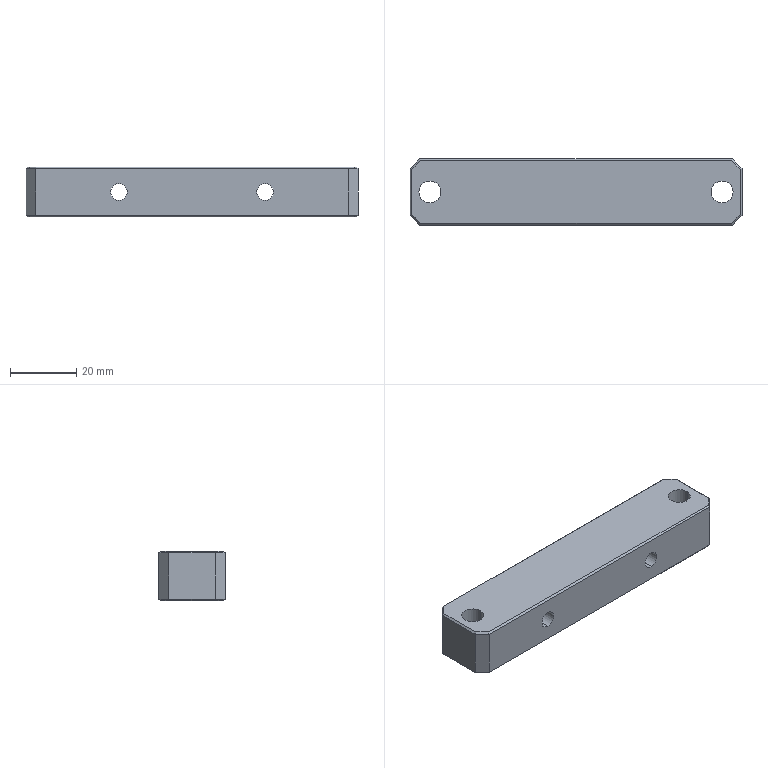Part | SolidWorks | features Chamfer 2, HoleWzd 2, Extrusion 1 | 1 solid | 40 faces | box 100 x 20 x 15 mm | volume 27033 mm3 | plane 28 | cylinder 12 | commonest cylinder face diameters 5 x4 6.6 x4 11 x4
STEP:
#1=CARTESIAN_POINT('',(22.,20.,10.));
#2=VERTEX_POINT('',#1);
#3=CARTESIAN_POINT('',(22.,20.,5.));
#4=VERTEX_POINT('',#3);
#5=CARTESIAN_POINT('',(22.,20.,7.5));
#6=DIRECTION('',(0.,-1.,0.));
#7=DIRECTION('',(0.,0.,-1.));
#8=AXIS2_PLACEMENT_3D('',#5,#6,#7);
#9=CIRCLE('',#8,2.5);
#10=EDGE_CURVE('',#2,#4,#9,.T.);
#11=ORIENTED_EDGE('',*,*,#10,.F.);
#12=CARTESIAN_POINT('',(22.,0.,10.));
#13=VERTEX_POINT('',#12);
#14=CARTESIAN_POINT('',(22.,0.,10.));
#15=DIRECTION('',(0.,-1.,0.));
#16=VECTOR('',#15,1000.);
#17=LINE('',#14,#16);
#18=EDGE_CURVE('',#2,#13,#17,.T.);
#19=ORIENTED_EDGE('',*,*,#18,.T.);
#20=CARTESIAN_POINT('',(22.,0.,5.));
#21=VERTEX_POINT('',#20);
#22=CARTESIAN_POINT('',(22.,0.,7.5));
#23=DIRECTION('',(0.,-1.,0.));
#24=DIRECTION('',(0.,0.,-1.));
#25=AXIS2_PLACEMENT_3D('',#22,#23,#24);
#26=CIRCLE('',#25,2.5);
#27=EDGE_CURVE('',#13,#21,#26,.T.);
#28=ORIENTED_EDGE('',*,*,#27,.T.);
#29=CARTESIAN_POINT('',(22.,0.,5.));
#30=DIRECTION('',(0.,-1.,0.));
#31=VECTOR('',#30,1000.);
#32=LINE('',#29,#31);
#33=EDGE_CURVE('',#4,#21,#32,.T.);
#34=ORIENTED_EDGE('',*,*,#33,.F.);
#35=EDGE_LOOP('',(#11,#19,#28,#34));
#36=FACE_OUTER_BOUND('',#35,.T.);
#37=CARTESIAN_POINT('',(22.,0.,7.5));
#38=DIRECTION('',(0.,-1.,0.));
#39=DIRECTION('',(0.,0.,-1.));
#40=AXIS2_PLACEMENT_3D('',#37,#38,#39);
#41=CYLINDRICAL_SURFACE('',#40,2.5);
#42=ADVANCED_FACE('',(#36),#41,.F.);
#43=CARTESIAN_POINT('',(-22.,20.,10.));
#44=VERTEX_POINT('',#43);
#45=CARTESIAN_POINT('',(-22.,20.,5.));
#46=VERTEX_POINT('',#45);
#47=CARTESIAN_POINT('',(-22.,20.,7.5));
#48=DIRECTION('',(0.,-1.,0.));
#49=DIRECTION('',(0.,0.,-1.));
#50=AXIS2_PLACEMENT_3D('',#47,#48,#49);
#51=CIRCLE('',#50,2.5);
#52=EDGE_CURVE('',#44,#46,#51,.T.);
#53=ORIENTED_EDGE('',*,*,#52,.F.);
#54=CARTESIAN_POINT('',(-22.,0.,10.));
#55=VERTEX_POINT('',#54);
#56=CARTESIAN_POINT('',(-22.,0.,10.));
#57=DIRECTION('',(0.,-1.,0.));
#58=VECTOR('',#57,1000.);
#59=LINE('',#56,#58);
#60=EDGE_CURVE('',#44,#55,#59,.T.);
#61=ORIENTED_EDGE('',*,*,#60,.T.);
#62=CARTESIAN_POINT('',(-22.,0.,5.));
#63=VERTEX_POINT('',#62);
#64=CARTESIAN_POINT('',(-22.,0.,7.5));
#65=DIRECTION('',(0.,-1.,0.));
#66=DIRECTION('',(0.,0.,-1.));
#67=AXIS2_PLACEMENT_3D('',#64,#65,#66);
#68=CIRCLE('',#67,2.5);
#69=EDGE_CURVE('',#55,#63,#68,.T.);
#70=ORIENTED_EDGE('',*,*,#69,.T.);
#71=CARTESIAN_POINT('',(-22.,0.,5.));
#72=DIRECTION('',(0.,-1.,0.));
#73=VECTOR('',#72,1000.);
#74=LINE('',#71,#73);
#75=EDGE_CURVE('',#46,#63,#74,.T.);
#76=ORIENTED_EDGE('',*,*,#75,.F.);
#77=EDGE_LOOP('',(#53,#61,#70,#76));
#78=FACE_OUTER_BOUND('',#77,.T.);
#79=CARTESIAN_POINT('',(-22.,0.,7.5));
#80=DIRECTION('',(0.,-1.,0.));
#81=DIRECTION('',(0.,0.,-1.));
#82=AXIS2_PLACEMENT_3D('',#79,#80,#81);
#83=CYLINDRICAL_SURFACE('',#82,2.5);
#84=ADVANCED_FACE('',(#78),#83,.F.);
#85=CARTESIAN_POINT('',(-38.5,10.,6.8));
#86=VERTEX_POINT('',#85);
#87=CARTESIAN_POINT('',(-49.5,10.,6.8));
#88=VERTEX_POINT('',#87);
#89=CARTESIAN_POINT('',(-44.,10.,6.8));
#90=DIRECTION('',(0.,0.,-1.));
#91=DIRECTION('',(-1.,0.,0.));
#92=AXIS2_PLACEMENT_3D('',#89,#90,#91);
#93=CIRCLE('',#92,5.5);
#94=EDGE_CURVE('',#86,#88,#93,.T.);
#95=ORIENTED_EDGE('',*,*,#94,.F.);
#96=CARTESIAN_POINT('',(-38.5,10.,0.));
#97=VERTEX_POINT('',#96);
#98=CARTESIAN_POINT('',(-38.5,10.,0.));
#99=DIRECTION('',(0.,0.,-1.));
#100=VECTOR('',#99,1000.);
#101=LINE('',#98,#100);
#102=EDGE_CURVE('',#86,#97,#101,.T.);
#103=ORIENTED_EDGE('',*,*,#102,.T.);
#104=CARTESIAN_POINT('',(-49.5,10.,0.));
#105=VERTEX_POINT('',#104);
#106=CARTESIAN_POINT('',(-44.,10.,0.));
#107=DIRECTION('',(0.,0.,-1.));
#108=DIRECTION('',(-1.,0.,0.));
#109=AXIS2_PLACEMENT_3D('',#106,#107,#108);
#110=CIRCLE('',#109,5.5);
#111=EDGE_CURVE('',#97,#105,#110,.T.);
#112=ORIENTED_EDGE('',*,*,#111,.T.);
#113=CARTESIAN_POINT('',(-49.5,10.,0.));
#114=DIRECTION('',(0.,0.,-1.));
#115=VECTOR('',#114,1000.);
#116=LINE('',#113,#115);
#117=EDGE_CURVE('',#88,#105,#116,.T.);
#118=ORIENTED_EDGE('',*,*,#117,.F.);
#119=EDGE_LOOP('',(#95,#103,#112,#118));
#120=FACE_OUTER_BOUND('',#119,.T.);
#121=CARTESIAN_POINT('',(-44.,10.,0.));
#122=DIRECTION('',(0.,0.,-1.));
#123=DIRECTION('',(-1.,0.,0.));
#124=AXIS2_PLACEMENT_3D('',#121,#122,#123);
#125=CYLINDRICAL_SURFACE('',#124,5.5);
#126=ADVANCED_FACE('',(#120),#125,.F.);
#127=CARTESIAN_POINT('',(-40.7,10.,15.));
#128=VERTEX_POINT('',#127);
#129=CARTESIAN_POINT('',(-47.3,10.,15.));
#130=VERTEX_POINT('',#129);
#131=CARTESIAN_POINT('',(-44.,10.,15.));
#132=DIRECTION('',(0.,0.,-1.));
#133=DIRECTION('',(-1.,0.,0.));
#134=AXIS2_PLACEMENT_3D('',#131,#132,#133);
#135=CIRCLE('',#134,3.3);
#136=EDGE_CURVE('',#128,#130,#135,.T.);
#137=ORIENTED_EDGE('',*,*,#136,.F.);
#138=CARTESIAN_POINT('',(-40.7,10.,6.8));
#139=VERTEX_POINT('',#138);
#140=CARTESIAN_POINT('',(-40.7,10.,0.));
#141=DIRECTION('',(0.,0.,-1.));
#142=VECTOR('',#141,1000.);
#143=LINE('',#140,#142);
#144=EDGE_CURVE('',#128,#139,#143,.T.);
#145=ORIENTED_EDGE('',*,*,#144,.T.);
#146=CARTESIAN_POINT('',(-47.3,10.,6.8));
#147=VERTEX_POINT('',#146);
#148=CARTESIAN_POINT('',(-44.,10.,6.8));
#149=DIRECTION('',(0.,0.,-1.));
#150=DIRECTION('',(-1.,0.,0.));
#151=AXIS2_PLACEMENT_3D('',#148,#149,#150);
#152=CIRCLE('',#151,3.3);
#153=EDGE_CURVE('',#139,#147,#152,.T.);
#154=ORIENTED_EDGE('',*,*,#153,.T.);
#155=CARTESIAN_POINT('',(-47.3,10.,0.));
#156=DIRECTION('',(0.,0.,-1.));
#157=VECTOR('',#156,1000.);
#158=LINE('',#155,#157);
#159=EDGE_CURVE('',#130,#147,#158,.T.);
#160=ORIENTED_EDGE('',*,*,#159,.F.);
#161=EDGE_LOOP('',(#137,#145,#154,#160));
#162=FACE_OUTER_BOUND('',#161,.T.);
#163=CARTESIAN_POINT('',(-44.,10.,0.));
#164=DIRECTION('',(0.,0.,-1.));
#165=DIRECTION('',(-1.,0.,0.));
#166=AXIS2_PLACEMENT_3D('',#163,#164,#165);
#167=CYLINDRICAL_SURFACE('',#166,3.3);
#168=ADVANCED_FACE('',(#162),#167,.F.);
#169=CARTESIAN_POINT('',(49.5,10.,6.8));
#170=VERTEX_POINT('',#169);
#171=CARTESIAN_POINT('',(38.5,10.,6.8));
#172=VERTEX_POINT('',#171);
#173=CARTESIAN_POINT('',(44.,10.,6.8));
#174=DIRECTION('',(0.,0.,-1.));
#175=DIRECTION('',(-1.,0.,0.));
#176=AXIS2_PLACEMENT_3D('',#173,#174,#175);
#177=CIRCLE('',#176,5.5);
#178=EDGE_CURVE('',#170,#172,#177,.T.);
#179=ORIENTED_EDGE('',*,*,#178,.F.);
#180=CARTESIAN_POINT('',(49.5,10.,0.));
#181=VERTEX_POINT('',#180);
#182=CARTESIAN_POINT('',(49.5,10.,0.));
#183=DIRECTION('',(0.,0.,-1.));
#184=VECTOR('',#183,1000.);
#185=LINE('',#182,#184);
#186=EDGE_CURVE('',#170,#181,#185,.T.);
#187=ORIENTED_EDGE('',*,*,#186,.T.);
#188=CARTESIAN_POINT('',(38.5,10.,0.));
#189=VERTEX_POINT('',#188);
#190=CARTESIAN_POINT('',(44.,10.,0.));
#191=DIRECTION('',(0.,0.,-1.));
#192=DIRECTION('',(-1.,0.,0.));
#193=AXIS2_PLACEMENT_3D('',#190,#191,#192);
#194=CIRCLE('',#193,5.5);
#195=EDGE_CURVE('',#181,#189,#194,.T.);
#196=ORIENTED_EDGE('',*,*,#195,.T.);
#197=CARTESIAN_POINT('',(38.5,10.,0.));
#198=DIRECTION('',(0.,0.,-1.));
#199=VECTOR('',#198,1000.);
#200=LINE('',#197,#199);
#201=EDGE_CURVE('',#172,#189,#200,.T.);
#202=ORIENTED_EDGE('',*,*,#201,.F.);
#203=EDGE_LOOP('',(#179,#187,#196,#202));
#204=FACE_OUTER_BOUND('',#203,.T.);
#205=CARTESIAN_POINT('',(44.,10.,0.));
#206=DIRECTION('',(0.,0.,-1.));
#207=DIRECTION('',(-1.,0.,0.));
#208=AXIS2_PLACEMENT_3D('',#205,#206,#207);
#209=CYLINDRICAL_SURFACE('',#208,5.5);
#210=ADVANCED_FACE('',(#204),#209,.F.);
#211=CARTESIAN_POINT('',(47.3,10.,15.));
#212=VERTEX_POINT('',#211);
#213=CARTESIAN_POINT('',(40.7,10.,15.));
#214=VERTEX_POINT('',#213);
#215=CARTESIAN_POINT('',(44.,10.,15.));
#216=DIRECTION('',(0.,0.,-1.));
#217=DIRECTION('',(-1.,0.,0.));
#218=AXIS2_PLACEMENT_3D('',#215,#216,#217);
#219=CIRCLE('',#218,3.3);
#220=EDGE_CURVE('',#212,#214,#219,.T.);
#221=ORIENTED_EDGE('',*,*,#220,.F.);
#222=CARTESIAN_POINT('',(47.3,10.,6.8));
#223=VERTEX_POINT('',#222);
#224=CARTESIAN_POINT('',(47.3,10.,0.));
#225=DIRECTION('',(0.,0.,-1.));
#226=VECTOR('',#225,1000.);
#227=LINE('',#224,#226);
#228=EDGE_CURVE('',#212,#223,#227,.T.);
#229=ORIENTED_EDGE('',*,*,#228,.T.);
#230=CARTESIAN_POINT('',(40.7,10.,6.8));
#231=VERTEX_POINT('',#230);
#232=CARTESIAN_POINT('',(44.,10.,6.8));
#233=DIRECTION('',(0.,0.,-1.));
#234=DIRECTION('',(-1.,0.,0.));
#235=AXIS2_PLACEMENT_3D('',#232,#233,#234);
#236=CIRCLE('',#235,3.3);
#237=EDGE_CURVE('',#223,#231,#236,.T.);
#238=ORIENTED_EDGE('',*,*,#237,.T.);
#239=CARTESIAN_POINT('',(40.7,10.,0.));
#240=DIRECTION('',(0.,0.,-1.));
#241=VECTOR('',#240,1000.);
#242=LINE('',#239,#241);
#243=EDGE_CURVE('',#214,#231,#242,.T.);
#244=ORIENTED_EDGE('',*,*,#243,.F.);
#245=EDGE_LOOP('',(#221,#229,#238,#244));
#246=FACE_OUTER_BOUND('',#245,.T.);
#247=CARTESIAN_POINT('',(44.,10.,0.));
#248=DIRECTION('',(0.,0.,-1.));
#249=DIRECTION('',(-1.,0.,0.));
#250=AXIS2_PLACEMENT_3D('',#247,#248,#249);
#251=CYLINDRICAL_SURFACE('',#250,3.3);
#252=ADVANCED_FACE('',(#246),#251,.F.);
#253=CARTESIAN_POINT('',(-50.,3.,0.5));
#254=VERTEX_POINT('',#253);
#255=CARTESIAN_POINT('',(-50.,3.,14.5));
#256=VERTEX_POINT('',#255);
#257=CARTESIAN_POINT('',(-50.,3.,15.));
#258=DIRECTION('',(0.,0.,1.));
#259=VECTOR('',#258,1000.);
#260=LINE('',#257,#259);
#261=EDGE_CURVE('',#254,#256,#260,.T.);
#262=ORIENTED_EDGE('',*,*,#261,.T.);
#263=CARTESIAN_POINT('',(-50.,17.,14.5));
#264=VERTEX_POINT('',#263);
#265=CARTESIAN_POINT('',(-50.,17.,14.5));
#266=DIRECTION('',(0.,1.,0.));
#267=VECTOR('',#266,1000.);
#268=LINE('',#265,#267);
#269=EDGE_CURVE('',#256,#264,#268,.T.);
#270=ORIENTED_EDGE('',*,*,#269,.T.);
#271=CARTESIAN_POINT('',(-50.,17.,0.5));
#272=VERTEX_POINT('',#271);
#273=CARTESIAN_POINT('',(-50.,17.,15.));
#274=DIRECTION('',(0.,0.,-1.));
#275=VECTOR('',#274,1000.);
#276=LINE('',#273,#275);
#277=EDGE_CURVE('',#264,#272,#276,.T.);
#278=ORIENTED_EDGE('',*,*,#277,.T.);
#279=CARTESIAN_POINT('',(-50.,20.,0.5));
#280=DIRECTION('',(0.,-1.,0.));
#281=VECTOR('',#280,1000.);
#282=LINE('',#279,#281);
#283=EDGE_CURVE('',#272,#254,#282,.T.);
#284=ORIENTED_EDGE('',*,*,#283,.T.);
#285=EDGE_LOOP('',(#262,#270,#278,#284));
#286=FACE_OUTER_BOUND('',#285,.T.);
#287=CARTESIAN_POINT('',(-50.,20.,15.));
#288=DIRECTION('',(1.,0.,0.));
#289=DIRECTION('',(0.,0.,-1.));
#290=AXIS2_PLACEMENT_3D('',#287,#288,#289);
#291=PLANE('',#290);
#292=ADVANCED_FACE('',(#286),#291,.F.);
#293=CARTESIAN_POINT('',(22.,0.,7.5));
#294=DIRECTION('',(0.,-1.,0.));
#295=DIRECTION('',(0.,0.,-1.));
#296=AXIS2_PLACEMENT_3D('',#293,#294,#295);
#297=CIRCLE('',#296,2.5);
#298=EDGE_CURVE('',#21,#13,#297,.T.);
#299=ORIENTED_EDGE('',*,*,#298,.F.);
#300=ORIENTED_EDGE('',*,*,#27,.F.);
#301=EDGE_LOOP('',(#299,#300));
#302=FACE_BOUND('',#301,.T.);
#303=CARTESIAN_POINT('',(-22.,0.,7.5));
#304=DIRECTION('',(0.,-1.,0.));
#305=DIRECTION('',(0.,0.,-1.));
#306=AXIS2_PLACEMENT_3D('',#303,#304,#305);
#307=CIRCLE('',#306,2.5);
#308=EDGE_CURVE('',#63,#55,#307,.T.);
#309=ORIENTED_EDGE('',*,*,#308,.F.);
#310=ORIENTED_EDGE('',*,*,#69,.F.);
#311=EDGE_LOOP('',(#309,#310));
#312=FACE_BOUND('',#311,.T.);
#313=CARTESIAN_POINT('',(47.,0.,0.5));
#314=VERTEX_POINT('',#313);
#315=CARTESIAN_POINT('',(47.,0.,14.5));
#316=VERTEX_POINT('',#315);
#317=CARTESIAN_POINT('',(47.,0.,15.));
#318=DIRECTION('',(0.,0.,1.));
#319=VECTOR('',#318,1000.);
#320=LINE('',#317,#319);
#321=EDGE_CURVE('',#314,#316,#320,.T.);
#322=ORIENTED_EDGE('',*,*,#321,.T.);
#323=CARTESIAN_POINT('',(-47.,0.,14.5));
#324=VERTEX_POINT('',#323);
#325=CARTESIAN_POINT('',(-47.,0.,14.5));
#326=DIRECTION('',(-1.,0.,0.));
#327=VECTOR('',#326,1000.);
#328=LINE('',#325,#327);
#329=EDGE_CURVE('',#316,#324,#328,.T.);
#330=ORIENTED_EDGE('',*,*,#329,.T.);
#331=CARTESIAN_POINT('',(-47.,0.,0.5));
#332=VERTEX_POINT('',#331);
#333=CARTESIAN_POINT('',(-47.,0.,15.));
#334=DIRECTION('',(0.,0.,-1.));
#335=VECTOR('',#334,1000.);
#336=LINE('',#333,#335);
#337=EDGE_CURVE('',#324,#332,#336,.T.);
#338=ORIENTED_EDGE('',*,*,#337,.T.);
#339=CARTESIAN_POINT('',(-50.,0.,0.5));
#340=DIRECTION('',(1.,0.,0.));
#341=VECTOR('',#340,1000.);
#342=LINE('',#339,#341);
#343=EDGE_CURVE('',#332,#314,#342,.T.);
#344=ORIENTED_EDGE('',*,*,#343,.T.);
#345=EDGE_LOOP('',(#322,#330,#338,#344));
#346=FACE_OUTER_BOUND('',#345,.T.);
#347=CARTESIAN_POINT('',(-50.,0.,15.));
#348=DIRECTION('',(0.,1.,0.));
#349=DIRECTION('',(0.,0.,1.));
#350=AXIS2_PLACEMENT_3D('',#347,#348,#349);
#351=PLANE('',#350);
#352=ADVANCED_FACE('',(#302,#312,#346),#351,.F.);
#353=CARTESIAN_POINT('',(50.,17.,0.5));
#354=VERTEX_POINT('',#353);
#355=CARTESIAN_POINT('',(50.,17.,14.5));
#356=VERTEX_POINT('',#355);
#357=CARTESIAN_POINT('',(50.,17.,15.));
#358=DIRECTION('',(0.,0.,1.));
#359=VECTOR('',#358,1000.);
#360=LINE('',#357,#359);
#361=EDGE_CURVE('',#354,#356,#360,.T.);
#362=ORIENTED_EDGE('',*,*,#361,.T.);
#363=CARTESIAN_POINT('',(50.,3.,14.5));
#364=VERTEX_POINT('',#363);
#365=CARTESIAN_POINT('',(50.,3.,14.5));
#366=DIRECTION('',(0.,-1.,0.));
#367=VECTOR('',#366,1000.);
#368=LINE('',#365,#367);
#369=EDGE_CURVE('',#356,#364,#368,.T.);
#370=ORIENTED_EDGE('',*,*,#369,.T.);
#371=CARTESIAN_POINT('',(50.,3.,0.5));
#372=VERTEX_POINT('',#371);
#373=CARTESIAN_POINT('',(50.,3.,15.));
#374=DIRECTION('',(0.,0.,-1.));
#375=VECTOR('',#374,1000.);
#376=LINE('',#373,#375);
#377=EDGE_CURVE('',#364,#372,#376,.T.);
#378=ORIENTED_EDGE('',*,*,#377,.T.);
#379=CARTESIAN_POINT('',(50.,20.,0.5));
#380=DIRECTION('',(0.,1.,0.));
#381=VECTOR('',#380,1000.);
#382=LINE('',#379,#381);
#383=EDGE_CURVE('',#372,#354,#382,.T.);
#384=ORIENTED_EDGE('',*,*,#383,.T.);
#385=EDGE_LOOP('',(#362,#370,#378,#384));
#386=FACE_OUTER_BOUND('',#385,.T.);
#387=CARTESIAN_POINT('',(50.,20.,15.));
#388=DIRECTION('',(-1.,0.,0.));
#389=DIRECTION('',(0.,0.,1.));
#390=AXIS2_PLACEMENT_3D('',#387,#388,#389);
#391=PLANE('',#390);
#392=ADVANCED_FACE('',(#386),#391,.F.);
#393=CARTESIAN_POINT('',(22.,20.,7.5));
#394=DIRECTION('',(0.,-1.,0.));
#395=DIRECTION('',(0.,0.,-1.));
#396=AXIS2_PLACEMENT_3D('',#393,#394,#395);
#397=CIRCLE('',#396,2.5);
#398=EDGE_CURVE('',#4,#2,#397,.T.);
#399=ORIENTED_EDGE('',*,*,#398,.T.);
#400=ORIENTED_EDGE('',*,*,#10,.T.);
#401=EDGE_LOOP('',(#399,#400));
#402=FACE_BOUND('',#401,.T.);
#403=CARTESIAN_POINT('',(-22.,20.,7.5));
#404=DIRECTION('',(0.,-1.,0.));
#405=DIRECTION('',(0.,0.,-1.));
#406=AXIS2_PLACEMENT_3D('',#403,#404,#405);
#407=CIRCLE('',#406,2.5);
#408=EDGE_CURVE('',#46,#44,#407,.T.);
#409=ORIENTED_EDGE('',*,*,#408,.T.);
#410=ORIENTED_EDGE('',*,*,#52,.T.);
#411=EDGE_LOOP('',(#409,#410));
#412=FACE_BOUND('',#411,.T.);
#413=CARTESIAN_POINT('',(-47.,20.,0.5));
#414=VERTEX_POINT('',#413);
#415=CARTESIAN_POINT('',(-47.,20.,14.5));
#416=VERTEX_POINT('',#415);
#417=CARTESIAN_POINT('',(-47.,20.,15.));
#418=DIRECTION('',(0.,0.,1.));
#419=VECTOR('',#418,1000.);
#420=LINE('',#417,#419);
#421=EDGE_CURVE('',#414,#416,#420,.T.);
#422=ORIENTED_EDGE('',*,*,#421,.T.);
#423=CARTESIAN_POINT('',(47.,20.,14.5));
#424=VERTEX_POINT('',#423);
#425=CARTESIAN_POINT('',(47.,20.,14.5));
#426=DIRECTION('',(1.,0.,0.));
#427=VECTOR('',#426,1000.);
#428=LINE('',#425,#427);
#429=EDGE_CURVE('',#416,#424,#428,.T.);
#430=ORIENTED_EDGE('',*,*,#429,.T.);
#431=CARTESIAN_POINT('',(47.,20.,0.5));
#432=VERTEX_POINT('',#431);
#433=CARTESIAN_POINT('',(47.,20.,15.));
#434=DIRECTION('',(0.,0.,-1.));
#435=VECTOR('',#434,1000.);
#436=LINE('',#433,#435);
#437=EDGE_CURVE('',#424,#432,#436,.T.);
#438=ORIENTED_EDGE('',*,*,#437,.T.);
#439=CARTESIAN_POINT('',(-50.,20.,0.5));
#440=DIRECTION('',(-1.,0.,0.));
#441=VECTOR('',#440,1000.);
#442=LINE('',#439,#441);
#443=EDGE_CURVE('',#432,#414,#442,.T.);
#444=ORIENTED_EDGE('',*,*,#443,.T.);
#445=EDGE_LOOP('',(#422,#430,#438,#444));
#446=FACE_OUTER_BOUND('',#445,.T.);
#447=CARTESIAN_POINT('',(-50.,20.,15.));
#448=DIRECTION('',(0.,-1.,0.));
#449=DIRECTION('',(1.,0.,0.));
#450=AXIS2_PLACEMENT_3D('',#447,#448,#449);
#451=PLANE('',#450);
#452=ADVANCED_FACE('',(#402,#412,#446),#451,.F.);
#453=CARTESIAN_POINT('',(49.5,3.207,15.));
#454=VERTEX_POINT('',#453);
#455=CARTESIAN_POINT('',(49.5,16.793,15.));
#456=VERTEX_POINT('',#455);
#457=CARTESIAN_POINT('',(49.5,17.,15.));
#458=DIRECTION('',(0.,1.,0.));
#459=VECTOR('',#458,1000.);
#460=LINE('',#457,#459);
#461=EDGE_CURVE('',#454,#456,#460,.T.);
#462=ORIENTED_EDGE('',*,*,#461,.T.);
#463=CARTESIAN_POINT('',(46.793,19.5,15.));
#464=VERTEX_POINT('',#463);
#465=CARTESIAN_POINT('',(33.146,33.146,15.));
#466=DIRECTION('',(-0.7071,0.7071,0.));
#467=VECTOR('',#466,1000.);
#468=LINE('',#465,#467);
#469=EDGE_CURVE('',#456,#464,#468,.T.);
#470=ORIENTED_EDGE('',*,*,#469,.T.);
#471=CARTESIAN_POINT('',(-46.793,19.5,15.));
#472=VERTEX_POINT('',#471);
#473=CARTESIAN_POINT('',(-47.,19.5,15.));
#474=DIRECTION('',(-1.,0.,0.));
#475=VECTOR('',#474,1000.);
#476=LINE('',#473,#475);
#477=EDGE_CURVE('',#464,#472,#476,.T.);
#478=ORIENTED_EDGE('',*,*,#477,.T.);
#479=CARTESIAN_POINT('',(-49.5,16.793,15.));
#480=VERTEX_POINT('',#479);
#481=CARTESIAN_POINT('',(-33.146,33.146,15.));
#482=DIRECTION('',(-0.7071,-0.7071,0.));
#483=VECTOR('',#482,1000.);
#484=LINE('',#481,#483);
#485=EDGE_CURVE('',#472,#480,#484,.T.);
#486=ORIENTED_EDGE('',*,*,#485,.T.);
#487=CARTESIAN_POINT('',(-49.5,3.207,15.));
#488=VERTEX_POINT('',#487);
#489=CARTESIAN_POINT('',(-49.5,3.,15.));
#490=DIRECTION('',(0.,-1.,0.));
#491=VECTOR('',#490,1000.);
#492=LINE('',#489,#491);
#493=EDGE_CURVE('',#480,#488,#492,.T.);
#494=ORIENTED_EDGE('',*,*,#493,.T.);
#495=CARTESIAN_POINT('',(-46.793,0.5,15.));
#496=VERTEX_POINT('',#495);
#497=CARTESIAN_POINT('',(-23.146,-23.146,15.));
#498=DIRECTION('',(0.7071,-0.7071,0.));
#499=VECTOR('',#498,1000.);
#500=LINE('',#497,#499);
#501=EDGE_CURVE('',#488,#496,#500,.T.);
#502=ORIENTED_EDGE('',*,*,#501,.T.);
#503=CARTESIAN_POINT('',(46.793,0.5,15.));
#504=VERTEX_POINT('',#503);
#505=CARTESIAN_POINT('',(47.,0.5,15.));
#506=DIRECTION('',(1.,0.,0.));
#507=VECTOR('',#506,1000.);
#508=LINE('',#505,#507);
#509=EDGE_CURVE('',#496,#504,#508,.T.);
#510=ORIENTED_EDGE('',*,*,#509,.T.);
#511=CARTESIAN_POINT('',(23.146,-23.146,15.));
#512=DIRECTION('',(0.7071,0.7071,0.));
#513=VECTOR('',#512,1000.);
#514=LINE('',#511,#513);
#515=EDGE_CURVE('',#504,#454,#514,.T.);
#516=ORIENTED_EDGE('',*,*,#515,.T.);
#517=EDGE_LOOP('',(#462,#470,#478,#486,#494,#502,#510,#516));
#518=FACE_OUTER_BOUND('',#517,.T.);
#519=CARTESIAN_POINT('',(-44.,10.,15.));
#520=DIRECTION('',(0.,0.,-1.));
#521=DIRECTION('',(-1.,0.,0.));
#522=AXIS2_PLACEMENT_3D('',#519,#520,#521);
#523=CIRCLE('',#522,3.3);
#524=EDGE_CURVE('',#130,#128,#523,.T.);
#525=ORIENTED_EDGE('',*,*,#524,.T.);
#526=ORIENTED_EDGE('',*,*,#136,.T.);
#527=EDGE_LOOP('',(#525,#526));
#528=FACE_BOUND('',#527,.T.);
#529=CARTESIAN_POINT('',(44.,10.,15.));
#530=DIRECTION('',(0.,0.,-1.));
#531=DIRECTION('',(-1.,0.,0.));
#532=AXIS2_PLACEMENT_3D('',#529,#530,#531);
#533=CIRCLE('',#532,3.3);
#534=EDGE_CURVE('',#214,#212,#533,.T.);
#535=ORIENTED_EDGE('',*,*,#534,.T.);
#536=ORIENTED_EDGE('',*,*,#220,.T.);
#537=EDGE_LOOP('',(#535,#536));
#538=FACE_BOUND('',#537,.T.);
#539=CARTESIAN_POINT('',(0.,0.,15.));
#540=DIRECTION('',(0.,0.,1.));
#541=DIRECTION('',(1.,0.,0.));
#542=AXIS2_PLACEMENT_3D('',#539,#540,#541);
#543=PLANE('',#542);
#544=ADVANCED_FACE('',(#518,#528,#538),#543,.T.);
#545=CARTESIAN_POINT('',(-46.793,0.5,0.));
#546=VERTEX_POINT('',#545);
#547=CARTESIAN_POINT('',(-49.5,3.207,0.));
#548=VERTEX_POINT('',#547);
#549=CARTESIAN_POINT('',(-49.646,3.354,0.));
#550=DIRECTION('',(-0.7071,0.7071,0.));
#551=VECTOR('',#550,1000.);
#552=LINE('',#549,#551);
#553=EDGE_CURVE('',#546,#548,#552,.T.);
#554=ORIENTED_EDGE('',*,*,#553,.T.);
#555=CARTESIAN_POINT('',(-49.5,0.,0.));
#556=DIRECTION('',(0.,1.,0.));
#557=VECTOR('',#556,1000.);
#558=LINE('',#555,#557);
#559=EDGE_CURVE('',#548,#105,#558,.T.);
#560=ORIENTED_EDGE('',*,*,#559,.T.);
#561=ORIENTED_EDGE('',*,*,#111,.F.);
#562=CARTESIAN_POINT('',(-44.,10.,0.));
#563=DIRECTION('',(0.,0.,-1.));
#564=DIRECTION('',(-1.,0.,0.));
#565=AXIS2_PLACEMENT_3D('',#562,#563,#564);
#566=CIRCLE('',#565,5.5);
#567=EDGE_CURVE('',#105,#97,#566,.T.);
#568=ORIENTED_EDGE('',*,*,#567,.F.);
#569=CARTESIAN_POINT('',(-49.5,16.793,0.));
#570=VERTEX_POINT('',#569);
#571=CARTESIAN_POINT('',(-49.5,0.,0.));
#572=DIRECTION('',(0.,1.,0.));
#573=VECTOR('',#572,1000.);
#574=LINE('',#571,#573);
#575=EDGE_CURVE('',#105,#570,#574,.T.);
#576=ORIENTED_EDGE('',*,*,#575,.T.);
#577=CARTESIAN_POINT('',(-46.793,19.5,0.));
#578=VERTEX_POINT('',#577);
#579=CARTESIAN_POINT('',(-46.646,19.646,0.));
#580=DIRECTION('',(0.7071,0.7071,0.));
#581=VECTOR('',#580,1000.);
#582=LINE('',#579,#581);
#583=EDGE_CURVE('',#570,#578,#582,.T.);
#584=ORIENTED_EDGE('',*,*,#583,.T.);
#585=CARTESIAN_POINT('',(46.793,19.5,0.));
#586=VERTEX_POINT('',#585);
#587=CARTESIAN_POINT('',(0.,19.5,0.));
#588=DIRECTION('',(1.,0.,0.));
#589=VECTOR('',#588,1000.);
#590=LINE('',#587,#589);
#591=EDGE_CURVE('',#578,#586,#590,.T.);
#592=ORIENTED_EDGE('',*,*,#591,.T.);
#593=CARTESIAN_POINT('',(49.5,16.793,0.));
#594=VERTEX_POINT('',#593);
#595=CARTESIAN_POINT('',(49.646,16.646,0.));
#596=DIRECTION('',(0.7071,-0.7071,0.));
#597=VECTOR('',#596,1000.);
#598=LINE('',#595,#597);
#599=EDGE_CURVE('',#586,#594,#598,.T.);
#600=ORIENTED_EDGE('',*,*,#599,.T.);
#601=CARTESIAN_POINT('',(49.5,0.,0.));
#602=DIRECTION('',(0.,-1.,0.));
#603=VECTOR('',#602,1000.);
#604=LINE('',#601,#603);
#605=EDGE_CURVE('',#594,#181,#604,.T.);
#606=ORIENTED_EDGE('',*,*,#605,.T.);
#607=CARTESIAN_POINT('',(44.,10.,0.));
#608=DIRECTION('',(0.,0.,-1.));
#609=DIRECTION('',(-1.,0.,0.));
#610=AXIS2_PLACEMENT_3D('',#607,#608,#609);
#611=CIRCLE('',#610,5.5);
#612=EDGE_CURVE('',#189,#181,#611,.T.);
#613=ORIENTED_EDGE('',*,*,#612,.F.);
#614=ORIENTED_EDGE('',*,*,#195,.F.);
#615=CARTESIAN_POINT('',(49.5,3.207,0.));
#616=VERTEX_POINT('',#615);
#617=CARTESIAN_POINT('',(49.5,0.,0.));
#618=DIRECTION('',(0.,-1.,0.));
#619=VECTOR('',#618,1000.);
#620=LINE('',#617,#619);
#621=EDGE_CURVE('',#181,#616,#620,.T.);
#622=ORIENTED_EDGE('',*,*,#621,.T.);
#623=CARTESIAN_POINT('',(46.793,0.5,0.));
#624=VERTEX_POINT('',#623);
#625=CARTESIAN_POINT('',(46.646,0.3536,0.));
#626=DIRECTION('',(-0.7071,-0.7071,0.));
#627=VECTOR('',#626,1000.);
#628=LINE('',#625,#627);
#629=EDGE_CURVE('',#616,#624,#628,.T.);
#630=ORIENTED_EDGE('',*,*,#629,.T.);
#631=CARTESIAN_POINT('',(0.,0.5,0.));
#632=DIRECTION('',(-1.,0.,0.));
#633=VECTOR('',#632,1000.);
#634=LINE('',#631,#633);
#635=EDGE_CURVE('',#624,#546,#634,.T.);
#636=ORIENTED_EDGE('',*,*,#635,.T.);
#637=EDGE_LOOP('',(#554,#560,#561,#568,#576,#584,#592,#600,#606,#613,#614,#622,#630,#636));
#638=FACE_OUTER_BOUND('',#637,.T.);
#639=CARTESIAN_POINT('',(0.,0.,0.));
#640=DIRECTION('',(0.,0.,1.));
#641=DIRECTION('',(1.,0.,0.));
#642=AXIS2_PLACEMENT_3D('',#639,#640,#641);
#643=PLANE('',#642);
#644=ADVANCED_FACE('',(#638),#643,.F.);
#645=ORIENTED_EDGE('',*,*,#228,.F.);
#646=ORIENTED_EDGE('',*,*,#534,.F.);
#647=ORIENTED_EDGE('',*,*,#243,.T.);
#648=CARTESIAN_POINT('',(44.,10.,6.8));
#649=DIRECTION('',(0.,0.,-1.));
#650=DIRECTION('',(-1.,0.,0.));
#651=AXIS2_PLACEMENT_3D('',#648,#649,#650);
#652=CIRCLE('',#651,3.3);
#653=EDGE_CURVE('',#231,#223,#652,.T.);
#654=ORIENTED_EDGE('',*,*,#653,.T.);
#655=EDGE_LOOP('',(#645,#646,#647,#654));
#656=FACE_OUTER_BOUND('',#655,.T.);
#657=CARTESIAN_POINT('',(44.,10.,0.));
#658=DIRECTION('',(0.,0.,-1.));
#659=DIRECTION('',(-1.,0.,0.));
#660=AXIS2_PLACEMENT_3D('',#657,#658,#659);
#661=CYLINDRICAL_SURFACE('',#660,3.3);
#662=ADVANCED_FACE('',(#656),#661,.F.);
#663=ORIENTED_EDGE('',*,*,#653,.F.);
#664=ORIENTED_EDGE('',*,*,#237,.F.);
#665=EDGE_LOOP('',(#663,#664));
#666=FACE_BOUND('',#665,.T.);
#667=CARTESIAN_POINT('',(44.,10.,6.8));
#668=DIRECTION('',(0.,0.,-1.));
#669=DIRECTION('',(-1.,0.,0.));
#670=AXIS2_PLACEMENT_3D('',#667,#668,#669);
#671=CIRCLE('',#670,5.5);
#672=EDGE_CURVE('',#172,#170,#671,.T.);
#673=ORIENTED_EDGE('',*,*,#672,.T.);
#674=ORIENTED_EDGE('',*,*,#178,.T.);
#675=EDGE_LOOP('',(#673,#674));
#676=FACE_OUTER_BOUND('',#675,.T.);
#677=CARTESIAN_POINT('',(47.3,10.,6.8));
#678=DIRECTION('',(0.,0.,1.));
#679=DIRECTION('',(1.,0.,0.));
#680=AXIS2_PLACEMENT_3D('',#677,#678,#679);
#681=PLANE('',#680);
#682=ADVANCED_FACE('',(#666,#676),#681,.F.);
#683=ORIENTED_EDGE('',*,*,#186,.F.);
#684=ORIENTED_EDGE('',*,*,#672,.F.);
#685=ORIENTED_EDGE('',*,*,#201,.T.);
#686=ORIENTED_EDGE('',*,*,#612,.T.);
#687=EDGE_LOOP('',(#683,#684,#685,#686));
#688=FACE_OUTER_BOUND('',#687,.T.);
#689=CARTESIAN_POINT('',(44.,10.,0.));
#690=DIRECTION('',(0.,0.,-1.));
#691=DIRECTION('',(-1.,0.,0.));
#692=AXIS2_PLACEMENT_3D('',#689,#690,#691);
#693=CYLINDRICAL_SURFACE('',#692,5.5);
#694=ADVANCED_FACE('',(#688),#693,.F.);
#695=ORIENTED_EDGE('',*,*,#144,.F.);
#696=ORIENTED_EDGE('',*,*,#524,.F.);
#697=ORIENTED_EDGE('',*,*,#159,.T.);
#698=CARTESIAN_POINT('',(-44.,10.,6.8));
#699=DIRECTION('',(0.,0.,-1.));
#700=DIRECTION('',(-1.,0.,0.));
#701=AXIS2_PLACEMENT_3D('',#698,#699,#700);
#702=CIRCLE('',#701,3.3);
#703=EDGE_CURVE('',#147,#139,#702,.T.);
#704=ORIENTED_EDGE('',*,*,#703,.T.);
#705=EDGE_LOOP('',(#695,#696,#697,#704));
#706=FACE_OUTER_BOUND('',#705,.T.);
#707=CARTESIAN_POINT('',(-44.,10.,0.));
#708=DIRECTION('',(0.,0.,-1.));
#709=DIRECTION('',(-1.,0.,0.));
#710=AXIS2_PLACEMENT_3D('',#707,#708,#709);
#711=CYLINDRICAL_SURFACE('',#710,3.3);
#712=ADVANCED_FACE('',(#706),#711,.F.);
#713=ORIENTED_EDGE('',*,*,#703,.F.);
#714=ORIENTED_EDGE('',*,*,#153,.F.);
#715=EDGE_LOOP('',(#713,#714));
#716=FACE_BOUND('',#715,.T.);
#717=CARTESIAN_POINT('',(-44.,10.,6.8));
#718=DIRECTION('',(0.,0.,-1.));
#719=DIRECTION('',(-1.,0.,0.));
#720=AXIS2_PLACEMENT_3D('',#717,#718,#719);
#721=CIRCLE('',#720,5.5);
#722=EDGE_CURVE('',#88,#86,#721,.T.);
#723=ORIENTED_EDGE('',*,*,#722,.T.);
#724=ORIENTED_EDGE('',*,*,#94,.T.);
#725=EDGE_LOOP('',(#723,#724));
#726=FACE_OUTER_BOUND('',#725,.T.);
#727=CARTESIAN_POINT('',(-40.7,10.,6.8));
#728=DIRECTION('',(0.,0.,1.));
#729=DIRECTION('',(1.,0.,0.));
#730=AXIS2_PLACEMENT_3D('',#727,#728,#729);
#731=PLANE('',#730);
#732=ADVANCED_FACE('',(#716,#726),#731,.F.);
#733=ORIENTED_EDGE('',*,*,#102,.F.);
#734=ORIENTED_EDGE('',*,*,#722,.F.);
#735=ORIENTED_EDGE('',*,*,#117,.T.);
#736=ORIENTED_EDGE('',*,*,#567,.T.);
#737=EDGE_LOOP('',(#733,#734,#735,#736));
#738=FACE_OUTER_BOUND('',#737,.T.);
#739=CARTESIAN_POINT('',(-44.,10.,0.));
#740=DIRECTION('',(0.,0.,-1.));
#741=DIRECTION('',(-1.,0.,0.));
#742=AXIS2_PLACEMENT_3D('',#739,#740,#741);
#743=CYLINDRICAL_SURFACE('',#742,5.5);
#744=ADVANCED_FACE('',(#738),#743,.F.);
#745=ORIENTED_EDGE('',*,*,#60,.F.);
#746=ORIENTED_EDGE('',*,*,#408,.F.);
#747=ORIENTED_EDGE('',*,*,#75,.T.);
#748=ORIENTED_EDGE('',*,*,#308,.T.);
#749=EDGE_LOOP('',(#745,#746,#747,#748));
#750=FACE_OUTER_BOUND('',#749,.T.);
#751=CARTESIAN_POINT('',(-22.,0.,7.5));
#752=DIRECTION('',(0.,-1.,0.));
#753=DIRECTION('',(0.,0.,-1.));
#754=AXIS2_PLACEMENT_3D('',#751,#752,#753);
#755=CYLINDRICAL_SURFACE('',#754,2.5);
#756=ADVANCED_FACE('',(#750),#755,.F.);
#757=ORIENTED_EDGE('',*,*,#18,.F.);
#758=ORIENTED_EDGE('',*,*,#398,.F.);
#759=ORIENTED_EDGE('',*,*,#33,.T.);
#760=ORIENTED_EDGE('',*,*,#298,.T.);
#761=EDGE_LOOP('',(#757,#758,#759,#760));
#762=FACE_OUTER_BOUND('',#761,.T.);
#763=CARTESIAN_POINT('',(22.,0.,7.5));
#764=DIRECTION('',(0.,-1.,0.));
#765=DIRECTION('',(0.,0.,-1.));
#766=AXIS2_PLACEMENT_3D('',#763,#764,#765);
#767=CYLINDRICAL_SURFACE('',#766,2.5);
#768=ADVANCED_FACE('',(#762),#767,.F.);
#769=ORIENTED_EDGE('',*,*,#337,.F.);
#770=CARTESIAN_POINT('',(-47.,0.,14.5));
#771=DIRECTION('',(-0.7071,0.7071,0.));
#772=VECTOR('',#771,1000.);
#773=LINE('',#770,#772);
#774=EDGE_CURVE('',#324,#256,#773,.T.);
#775=ORIENTED_EDGE('',*,*,#774,.T.);
#776=ORIENTED_EDGE('',*,*,#261,.F.);
#777=CARTESIAN_POINT('',(-47.,0.,0.5));
#778=DIRECTION('',(0.7071,-0.7071,0.));
#779=VECTOR('',#778,1000.);
#780=LINE('',#777,#779);
#781=EDGE_CURVE('',#254,#332,#780,.T.);
#782=ORIENTED_EDGE('',*,*,#781,.T.);
#783=EDGE_LOOP('',(#769,#775,#776,#782));
#784=FACE_OUTER_BOUND('',#783,.T.);
#785=CARTESIAN_POINT('',(-47.,0.,15.));
#786=DIRECTION('',(0.7071,0.7071,0.));
#787=DIRECTION('',(0.,0.,-1.));
#788=AXIS2_PLACEMENT_3D('',#785,#786,#787);
#789=PLANE('',#788);
#790=ADVANCED_FACE('',(#784),#789,.F.);
#791=ORIENTED_EDGE('',*,*,#277,.F.);
#792=CARTESIAN_POINT('',(-50.,17.,14.5));
#793=DIRECTION('',(0.7071,0.7071,0.));
#794=VECTOR('',#793,1000.);
#795=LINE('',#792,#794);
#796=EDGE_CURVE('',#264,#416,#795,.T.);
#797=ORIENTED_EDGE('',*,*,#796,.T.);
#798=ORIENTED_EDGE('',*,*,#421,.F.);
#799=CARTESIAN_POINT('',(-50.,17.,0.5));
#800=DIRECTION('',(-0.7071,-0.7071,0.));
#801=VECTOR('',#800,1000.);
#802=LINE('',#799,#801);
#803=EDGE_CURVE('',#414,#272,#802,.T.);
#804=ORIENTED_EDGE('',*,*,#803,.T.);
#805=EDGE_LOOP('',(#791,#797,#798,#804));
#806=FACE_OUTER_BOUND('',#805,.T.);
#807=CARTESIAN_POINT('',(-50.,17.,15.));
#808=DIRECTION('',(0.7071,-0.7071,0.));
#809=DIRECTION('',(0.,0.,-1.));
#810=AXIS2_PLACEMENT_3D('',#807,#808,#809);
#811=PLANE('',#810);
#812=ADVANCED_FACE('',(#806),#811,.F.);
#813=ORIENTED_EDGE('',*,*,#377,.F.);
#814=CARTESIAN_POINT('',(50.,3.,14.5));
#815=DIRECTION('',(-0.7071,-0.7071,0.));
#816=VECTOR('',#815,1000.);
#817=LINE('',#814,#816);
#818=EDGE_CURVE('',#364,#316,#817,.T.);
#819=ORIENTED_EDGE('',*,*,#818,.T.);
#820=ORIENTED_EDGE('',*,*,#321,.F.);
#821=CARTESIAN_POINT('',(50.,3.,0.5));
#822=DIRECTION('',(0.7071,0.7071,0.));
#823=VECTOR('',#822,1000.);
#824=LINE('',#821,#823);
#825=EDGE_CURVE('',#314,#372,#824,.T.);
#826=ORIENTED_EDGE('',*,*,#825,.T.);
#827=EDGE_LOOP('',(#813,#819,#820,#826));
#828=FACE_OUTER_BOUND('',#827,.T.);
#829=CARTESIAN_POINT('',(50.,3.,15.));
#830=DIRECTION('',(-0.7071,0.7071,0.));
#831=DIRECTION('',(0.,0.,-1.));
#832=AXIS2_PLACEMENT_3D('',#829,#830,#831);
#833=PLANE('',#832);
#834=ADVANCED_FACE('',(#828),#833,.F.);
#835=ORIENTED_EDGE('',*,*,#437,.F.);
#836=CARTESIAN_POINT('',(47.,20.,14.5));
#837=DIRECTION('',(0.7071,-0.7071,0.));
#838=VECTOR('',#837,1000.);
#839=LINE('',#836,#838);
#840=EDGE_CURVE('',#424,#356,#839,.T.);
#841=ORIENTED_EDGE('',*,*,#840,.T.);
#842=ORIENTED_EDGE('',*,*,#361,.F.);
#843=CARTESIAN_POINT('',(47.,20.,0.5));
#844=DIRECTION('',(-0.7071,0.7071,0.));
#845=VECTOR('',#844,1000.);
#846=LINE('',#843,#845);
#847=EDGE_CURVE('',#354,#432,#846,.T.);
#848=ORIENTED_EDGE('',*,*,#847,.T.);
#849=EDGE_LOOP('',(#835,#841,#842,#848));
#850=FACE_OUTER_BOUND('',#849,.T.);
#851=CARTESIAN_POINT('',(47.,20.,15.));
#852=DIRECTION('',(-0.7071,-0.7071,0.));
#853=DIRECTION('',(0.,0.,-1.));
#854=AXIS2_PLACEMENT_3D('',#851,#852,#853);
#855=PLANE('',#854);
#856=ADVANCED_FACE('',(#850),#855,.F.);
#857=CARTESIAN_POINT('',(-50.112,2.954,14.388));
#858=DIRECTION('',(0.6786,0.2811,0.6786));
#859=VECTOR('',#858,1000.);
#860=LINE('',#857,#859);
#861=EDGE_CURVE('',#256,#488,#860,.T.);
#862=ORIENTED_EDGE('',*,*,#861,.F.);
#863=ORIENTED_EDGE('',*,*,#774,.F.);
#864=CARTESIAN_POINT('',(-49.435,-5.879,8.621));
#865=DIRECTION('',(-0.2811,-0.6786,-0.6786));
#866=VECTOR('',#865,1000.);
#867=LINE('',#864,#866);
#868=EDGE_CURVE('',#496,#324,#867,.T.);
#869=ORIENTED_EDGE('',*,*,#868,.F.);
#870=ORIENTED_EDGE('',*,*,#501,.F.);
#871=EDGE_LOOP('',(#862,#863,#869,#870));
#872=FACE_OUTER_BOUND('',#871,.T.);
#873=CARTESIAN_POINT('',(-23.146,-23.146,15.));
#874=DIRECTION('',(-0.5,-0.5,0.7071));
#875=DIRECTION('',(-0.7071,0.7071,0.));
#876=AXIS2_PLACEMENT_3D('',#873,#874,#875);
#877=PLANE('',#876);
#878=ADVANCED_FACE('',(#872),#877,.T.);
#879=ORIENTED_EDGE('',*,*,#868,.T.);
#880=ORIENTED_EDGE('',*,*,#329,.F.);
#881=CARTESIAN_POINT('',(43.096,9.425,23.925));
#882=DIRECTION('',(0.2811,-0.6786,-0.6786));
#883=VECTOR('',#882,1000.);
#884=LINE('',#881,#883);
#885=EDGE_CURVE('',#504,#316,#884,.T.);
#886=ORIENTED_EDGE('',*,*,#885,.F.);
#887=ORIENTED_EDGE('',*,*,#509,.F.);
#888=EDGE_LOOP('',(#879,#880,#886,#887));
#889=FACE_OUTER_BOUND('',#888,.T.);
#890=CARTESIAN_POINT('',(0.,0.5,15.));
#891=DIRECTION('',(0.,-0.7071,0.7071));
#892=DIRECTION('',(-1.,0.,0.));
#893=AXIS2_PLACEMENT_3D('',#890,#891,#892);
#894=PLANE('',#893);
#895=ADVANCED_FACE('',(#889),#894,.T.);
#896=ORIENTED_EDGE('',*,*,#861,.T.);
#897=ORIENTED_EDGE('',*,*,#493,.F.);
#898=CARTESIAN_POINT('',(-45.089,14.966,19.411));
#899=DIRECTION('',(0.6786,-0.2811,0.6786));
#900=VECTOR('',#899,1000.);
#901=LINE('',#898,#900);
#902=EDGE_CURVE('',#264,#480,#901,.T.);
#903=ORIENTED_EDGE('',*,*,#902,.F.);
#904=ORIENTED_EDGE('',*,*,#269,.F.);
#905=EDGE_LOOP('',(#896,#897,#903,#904));
#906=FACE_OUTER_BOUND('',#905,.T.);
#907=CARTESIAN_POINT('',(-49.5,0.,15.));
#908=DIRECTION('',(-0.7071,0.,0.7071));
#909=DIRECTION('',(0.,1.,0.));
#910=AXIS2_PLACEMENT_3D('',#907,#908,#909);
#911=PLANE('',#910);
#912=ADVANCED_FACE('',(#906),#911,.T.);
#913=ORIENTED_EDGE('',*,*,#885,.T.);
#914=ORIENTED_EDGE('',*,*,#818,.F.);
#915=CARTESIAN_POINT('',(42.391,6.152,22.109));
#916=DIRECTION('',(0.6786,-0.2811,-0.6786));
#917=VECTOR('',#916,1000.);
#918=LINE('',#915,#917);
#919=EDGE_CURVE('',#454,#364,#918,.T.);
#920=ORIENTED_EDGE('',*,*,#919,.F.);
#921=ORIENTED_EDGE('',*,*,#515,.F.);
#922=EDGE_LOOP('',(#913,#914,#920,#921));
#923=FACE_OUTER_BOUND('',#922,.T.);
#924=CARTESIAN_POINT('',(23.146,-23.146,15.));
#925=DIRECTION('',(0.5,-0.5,0.7071));
#926=DIRECTION('',(-0.7071,-0.7071,0.));
#927=AXIS2_PLACEMENT_3D('',#924,#925,#926);
#928=PLANE('',#927);
#929=ADVANCED_FACE('',(#923),#928,.T.);
#930=ORIENTED_EDGE('',*,*,#902,.T.);
#931=ORIENTED_EDGE('',*,*,#485,.F.);
#932=CARTESIAN_POINT('',(-43.096,10.575,23.925));
#933=DIRECTION('',(0.2811,-0.6786,0.6786));
#934=VECTOR('',#933,1000.);
#935=LINE('',#932,#934);
#936=EDGE_CURVE('',#416,#472,#935,.T.);
#937=ORIENTED_EDGE('',*,*,#936,.F.);
#938=ORIENTED_EDGE('',*,*,#796,.F.);
#939=EDGE_LOOP('',(#930,#931,#937,#938));
#940=FACE_OUTER_BOUND('',#939,.T.);
#941=CARTESIAN_POINT('',(-33.146,33.146,15.));
#942=DIRECTION('',(-0.5,0.5,0.7071));
#943=DIRECTION('',(0.7071,0.7071,0.));
#944=AXIS2_PLACEMENT_3D('',#941,#942,#943);
#945=PLANE('',#944);
#946=ADVANCED_FACE('',(#940),#945,.T.);
#947=ORIENTED_EDGE('',*,*,#919,.T.);
#948=ORIENTED_EDGE('',*,*,#369,.F.);
#949=CARTESIAN_POINT('',(46.297,15.466,18.203));
#950=DIRECTION('',(0.6786,0.2811,-0.6786));
#951=VECTOR('',#950,1000.);
#952=LINE('',#949,#951);
#953=EDGE_CURVE('',#456,#356,#952,.T.);
#954=ORIENTED_EDGE('',*,*,#953,.F.);
#955=ORIENTED_EDGE('',*,*,#461,.F.);
#956=EDGE_LOOP('',(#947,#948,#954,#955));
#957=FACE_OUTER_BOUND('',#956,.T.);
#958=CARTESIAN_POINT('',(49.5,0.,15.));
#959=DIRECTION('',(0.7071,0.,0.7071));
#960=DIRECTION('',(0.,-1.,0.));
#961=AXIS2_PLACEMENT_3D('',#958,#959,#960);
#962=PLANE('',#961);
#963=ADVANCED_FACE('',(#957),#962,.T.);
#964=ORIENTED_EDGE('',*,*,#936,.T.);
#965=ORIENTED_EDGE('',*,*,#477,.F.);
#966=CARTESIAN_POINT('',(43.096,10.575,23.925));
#967=DIRECTION('',(-0.2811,-0.6786,0.6786));
#968=VECTOR('',#967,1000.);
#969=LINE('',#966,#968);
#970=EDGE_CURVE('',#424,#464,#969,.T.);
#971=ORIENTED_EDGE('',*,*,#970,.F.);
#972=ORIENTED_EDGE('',*,*,#429,.F.);
#973=EDGE_LOOP('',(#964,#965,#971,#972));
#974=FACE_OUTER_BOUND('',#973,.T.);
#975=CARTESIAN_POINT('',(0.,19.5,15.));
#976=DIRECTION('',(0.,0.7071,0.7071));
#977=DIRECTION('',(1.,0.,0.));
#978=AXIS2_PLACEMENT_3D('',#975,#976,#977);
#979=PLANE('',#978);
#980=ADVANCED_FACE('',(#974),#979,.T.);
#981=ORIENTED_EDGE('',*,*,#953,.T.);
#982=ORIENTED_EDGE('',*,*,#840,.F.);
#983=ORIENTED_EDGE('',*,*,#970,.T.);
#984=ORIENTED_EDGE('',*,*,#469,.F.);
#985=EDGE_LOOP('',(#981,#982,#983,#984));
#986=FACE_OUTER_BOUND('',#985,.T.);
#987=CARTESIAN_POINT('',(33.146,33.146,15.));
#988=DIRECTION('',(0.5,0.5,0.7071));
#989=DIRECTION('',(0.7071,-0.7071,0.));
#990=AXIS2_PLACEMENT_3D('',#987,#988,#989);
#991=PLANE('',#990);
#992=ADVANCED_FACE('',(#986),#991,.T.);
#993=CARTESIAN_POINT('',(46.757,4.343,-2.743));
#994=DIRECTION('',(-0.6786,0.2811,-0.6786));
#995=VECTOR('',#994,1000.);
#996=LINE('',#993,#995);
#997=EDGE_CURVE('',#372,#616,#996,.T.);
#998=ORIENTED_EDGE('',*,*,#997,.F.);
#999=ORIENTED_EDGE('',*,*,#825,.F.);
#1000=CARTESIAN_POINT('',(49.435,-5.879,6.379));
#1001=DIRECTION('',(0.2811,-0.6786,0.6786));
#1002=VECTOR('',#1001,1000.);
#1003=LINE('',#1000,#1002);
#1004=EDGE_CURVE('',#624,#314,#1003,.T.);
#1005=ORIENTED_EDGE('',*,*,#1004,.F.);
#1006=ORIENTED_EDGE('',*,*,#629,.F.);
#1007=EDGE_LOOP('',(#998,#999,#1005,#1006));
#1008=FACE_OUTER_BOUND('',#1007,.T.);
#1009=CARTESIAN_POINT('',(23.146,-23.146,0.));
#1010=DIRECTION('',(-0.5,0.5,0.7071));
#1011=DIRECTION('',(-0.7071,-0.7071,0.));
#1012=AXIS2_PLACEMENT_3D('',#1009,#1010,#1011);
#1013=PLANE('',#1012);
#1014=ADVANCED_FACE('',(#1008),#1013,.F.);
#1015=ORIENTED_EDGE('',*,*,#1004,.T.);
#1016=ORIENTED_EDGE('',*,*,#343,.F.);
#1017=CARTESIAN_POINT('',(-47.237,-0.5722,1.072));
#1018=DIRECTION('',(-0.2811,-0.6786,0.6786));
#1019=VECTOR('',#1018,1000.);
#1020=LINE('',#1017,#1019);
#1021=EDGE_CURVE('',#546,#332,#1020,.T.);
#1022=ORIENTED_EDGE('',*,*,#1021,.F.);
#1023=ORIENTED_EDGE('',*,*,#635,.F.);
#1024=EDGE_LOOP('',(#1015,#1016,#1022,#1023));
#1025=FACE_OUTER_BOUND('',#1024,.T.);
#1026=CARTESIAN_POINT('',(-50.,0.,0.5));
#1027=DIRECTION('',(0.,0.7071,0.7071));
#1028=DIRECTION('',(1.,0.,0.));
#1029=AXIS2_PLACEMENT_3D('',#1026,#1027,#1028);
#1030=PLANE('',#1029);
#1031=ADVANCED_FACE('',(#1025),#1030,.F.);
#1032=ORIENTED_EDGE('',*,*,#621,.F.);
#1033=ORIENTED_EDGE('',*,*,#605,.F.);
#1034=CARTESIAN_POINT('',(45.089,14.966,-4.411));
#1035=DIRECTION('',(-0.6786,-0.2811,-0.6786));
#1036=VECTOR('',#1035,1000.);
#1037=LINE('',#1034,#1036);
#1038=EDGE_CURVE('',#354,#594,#1037,.T.);
#1039=ORIENTED_EDGE('',*,*,#1038,.F.);
#1040=ORIENTED_EDGE('',*,*,#383,.F.);
#1041=ORIENTED_EDGE('',*,*,#997,.T.);
#1042=EDGE_LOOP('',(#1032,#1033,#1039,#1040,#1041));
#1043=FACE_OUTER_BOUND('',#1042,.T.);
#1044=CARTESIAN_POINT('',(50.,20.,0.5));
#1045=DIRECTION('',(-0.7071,0.,0.7071));
#1046=DIRECTION('',(0.,1.,0.));
#1047=AXIS2_PLACEMENT_3D('',#1044,#1045,#1046);
#1048=PLANE('',#1047);
#1049=ADVANCED_FACE('',(#1043),#1048,.F.);
#1050=ORIENTED_EDGE('',*,*,#1021,.T.);
#1051=ORIENTED_EDGE('',*,*,#781,.F.);
#1052=CARTESIAN_POINT('',(-42.391,6.152,-7.109));
#1053=DIRECTION('',(-0.6786,-0.2811,0.6786));
#1054=VECTOR('',#1053,1000.);
#1055=LINE('',#1052,#1054);
#1056=EDGE_CURVE('',#548,#254,#1055,.T.);
#1057=ORIENTED_EDGE('',*,*,#1056,.F.);
#1058=ORIENTED_EDGE('',*,*,#553,.F.);
#1059=EDGE_LOOP('',(#1050,#1051,#1057,#1058));
#1060=FACE_OUTER_BOUND('',#1059,.T.);
#1061=CARTESIAN_POINT('',(-23.146,-23.146,0.));
#1062=DIRECTION('',(0.5,0.5,0.7071));
#1063=DIRECTION('',(-0.7071,0.7071,0.));
#1064=AXIS2_PLACEMENT_3D('',#1061,#1062,#1063);
#1065=PLANE('',#1064);
#1066=ADVANCED_FACE('',(#1060),#1065,.F.);
#1067=ORIENTED_EDGE('',*,*,#1038,.T.);
#1068=ORIENTED_EDGE('',*,*,#599,.F.);
#1069=CARTESIAN_POINT('',(39.336,1.498,-18.002));
#1070=DIRECTION('',(-0.2811,-0.6786,-0.6786));
#1071=VECTOR('',#1070,1000.);
#1072=LINE('',#1069,#1071);
#1073=EDGE_CURVE('',#432,#586,#1072,.T.);
#1074=ORIENTED_EDGE('',*,*,#1073,.F.);
#1075=ORIENTED_EDGE('',*,*,#847,.F.);
#1076=EDGE_LOOP('',(#1067,#1068,#1074,#1075));
#1077=FACE_OUTER_BOUND('',#1076,.T.);
#1078=CARTESIAN_POINT('',(33.146,33.146,0.));
#1079=DIRECTION('',(-0.5,-0.5,0.7071));
#1080=DIRECTION('',(0.7071,-0.7071,0.));
#1081=AXIS2_PLACEMENT_3D('',#1078,#1079,#1080);
#1082=PLANE('',#1081);
#1083=ADVANCED_FACE('',(#1077),#1082,.F.);
#1084=ORIENTED_EDGE('',*,*,#1056,.T.);
#1085=ORIENTED_EDGE('',*,*,#283,.F.);
#1086=CARTESIAN_POINT('',(-50.572,17.237,1.072));
#1087=DIRECTION('',(-0.6786,0.2811,0.6786));
#1088=VECTOR('',#1087,1000.);
#1089=LINE('',#1086,#1088);
#1090=EDGE_CURVE('',#570,#272,#1089,.T.);
#1091=ORIENTED_EDGE('',*,*,#1090,.F.);
#1092=ORIENTED_EDGE('',*,*,#575,.F.);
#1093=ORIENTED_EDGE('',*,*,#559,.F.);
#1094=EDGE_LOOP('',(#1084,#1085,#1091,#1092,#1093));
#1095=FACE_OUTER_BOUND('',#1094,.T.);
#1096=CARTESIAN_POINT('',(-50.,20.,0.5));
#1097=DIRECTION('',(0.7071,0.,0.7071));
#1098=DIRECTION('',(0.,-1.,0.));
#1099=AXIS2_PLACEMENT_3D('',#1096,#1097,#1098);
#1100=PLANE('',#1099);
#1101=ADVANCED_FACE('',(#1095),#1100,.F.);
#1102=ORIENTED_EDGE('',*,*,#1073,.T.);
#1103=ORIENTED_EDGE('',*,*,#591,.F.);
#1104=CARTESIAN_POINT('',(-47.237,20.572,1.072));
#1105=DIRECTION('',(0.2811,-0.6786,-0.6786));
#1106=VECTOR('',#1105,1000.);
#1107=LINE('',#1104,#1106);
#1108=EDGE_CURVE('',#414,#578,#1107,.T.);
#1109=ORIENTED_EDGE('',*,*,#1108,.F.);
#1110=ORIENTED_EDGE('',*,*,#443,.F.);
#1111=EDGE_LOOP('',(#1102,#1103,#1109,#1110));
#1112=FACE_OUTER_BOUND('',#1111,.T.);
#1113=CARTESIAN_POINT('',(-50.,20.,0.5));
#1114=DIRECTION('',(0.,-0.7071,0.7071));
#1115=DIRECTION('',(-1.,0.,0.));
#1116=AXIS2_PLACEMENT_3D('',#1113,#1114,#1115);
#1117=PLANE('',#1116);
#1118=ADVANCED_FACE('',(#1112),#1117,.F.);
#1119=ORIENTED_EDGE('',*,*,#1090,.T.);
#1120=ORIENTED_EDGE('',*,*,#803,.F.);
#1121=ORIENTED_EDGE('',*,*,#1108,.T.);
#1122=ORIENTED_EDGE('',*,*,#583,.F.);
#1123=EDGE_LOOP('',(#1119,#1120,#1121,#1122));
#1124=FACE_OUTER_BOUND('',#1123,.T.);
#1125=CARTESIAN_POINT('',(-33.146,33.146,0.));
#1126=DIRECTION('',(0.5,-0.5,0.7071));
#1127=DIRECTION('',(0.7071,0.7071,0.));
#1128=AXIS2_PLACEMENT_3D('',#1125,#1126,#1127);
#1129=PLANE('',#1128);
#1130=ADVANCED_FACE('',(#1124),#1129,.F.);
#1131=CLOSED_SHELL('',(#42,#84,#126,#168,#210,#252,#292,#352,#392,#452,#544,#644,#662,#682,#694,#712,#732,#744,#756,#768,#790,#812,#834,#856,#878,#895,#912,#929,#946,#963,#980,#992,#1014,#1031,#1049,#1066,#1083,#1101,#1118,#1130));
#1132=MANIFOLD_SOLID_BREP('',#1131);
#1133=CARTESIAN_POINT('',(0.,0.,0.));
#1134=DIRECTION('',(0.,0.,1.));
#1135=DIRECTION('',(1.,0.,0.));
#1136=AXIS2_PLACEMENT_3D('',#1133,#1134,#1135);
#1137=(LENGTH_UNIT()NAMED_UNIT(*)SI_UNIT(.MILLI.,.METRE.));
#1138=UNCERTAINTY_MEASURE_WITH_UNIT(LENGTH_MEASURE(0.00001),#1137,'','');
#1139=(NAMED_UNIT(*)PLANE_ANGLE_UNIT()SI_UNIT($,.RADIAN.));
#1140=(NAMED_UNIT(*)SI_UNIT($,.STERADIAN.)SOLID_ANGLE_UNIT());
#1141=(GEOMETRIC_REPRESENTATION_CONTEXT(3)GLOBAL_UNCERTAINTY_ASSIGNED_CONTEXT((#1138))GLOBAL_UNIT_ASSIGNED_CONTEXT((#1137,#1139,#1140))REPRESENTATION_CONTEXT('',''));
#1142=ADVANCED_BREP_SHAPE_REPRESENTATION('',(#1132,#1136),#1141);